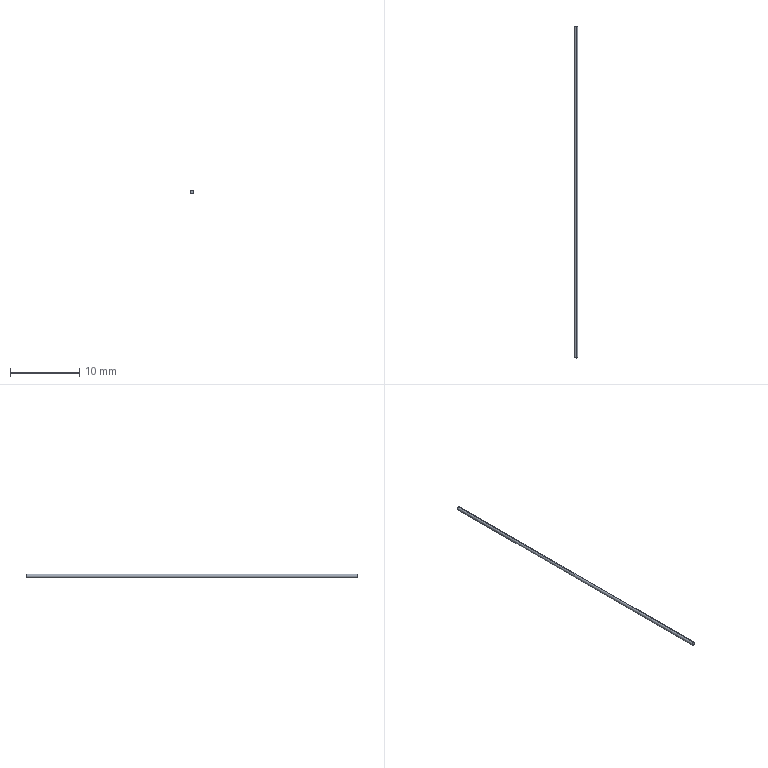Part | SolidWorks | features Revolution 1 | 1 solid | 4 faces | box 0.5 x 48 x 0.5 mm | volume 9.425 mm3 | cylinder 2 | plane 2 | commonest cylinder face diameters 0.5 x2
STEP:
#1=CARTESIAN_POINT('',(0.,48.,-0.25));
#2=VERTEX_POINT('',#1);
#3=CARTESIAN_POINT('',(0.,48.,0.25));
#4=VERTEX_POINT('',#3);
#5=CARTESIAN_POINT('',(0.,48.,0.));
#6=DIRECTION('',(0.,-1.,0.));
#7=DIRECTION('',(0.,0.,-1.));
#8=AXIS2_PLACEMENT_3D('',#5,#6,#7);
#9=CIRCLE('',#8,0.25);
#10=EDGE_CURVE('',#2,#4,#9,.T.);
#11=ORIENTED_EDGE('',*,*,#10,.T.);
#12=CARTESIAN_POINT('',(0.,0.,0.25));
#13=VERTEX_POINT('',#12);
#14=CARTESIAN_POINT('',(0.,0.,0.25));
#15=DIRECTION('',(0.,-1.,0.));
#16=VECTOR('',#15,1000.);
#17=LINE('',#14,#16);
#18=EDGE_CURVE('',#4,#13,#17,.T.);
#19=ORIENTED_EDGE('',*,*,#18,.T.);
#20=CARTESIAN_POINT('',(0.,0.,-0.25));
#21=VERTEX_POINT('',#20);
#22=CARTESIAN_POINT('',(0.,0.,0.));
#23=DIRECTION('',(0.,-1.,0.));
#24=DIRECTION('',(0.,0.,-1.));
#25=AXIS2_PLACEMENT_3D('',#22,#23,#24);
#26=CIRCLE('',#25,0.25);
#27=EDGE_CURVE('',#21,#13,#26,.T.);
#28=ORIENTED_EDGE('',*,*,#27,.F.);
#29=CARTESIAN_POINT('',(0.,0.,-0.25));
#30=DIRECTION('',(0.,-1.,0.));
#31=VECTOR('',#30,1000.);
#32=LINE('',#29,#31);
#33=EDGE_CURVE('',#2,#21,#32,.T.);
#34=ORIENTED_EDGE('',*,*,#33,.F.);
#35=EDGE_LOOP('',(#11,#19,#28,#34));
#36=FACE_OUTER_BOUND('',#35,.T.);
#37=CARTESIAN_POINT('',(0.,0.,0.));
#38=DIRECTION('',(0.,-1.,0.));
#39=DIRECTION('',(0.,0.,-1.));
#40=AXIS2_PLACEMENT_3D('',#37,#38,#39);
#41=CYLINDRICAL_SURFACE('',#40,0.25);
#42=ADVANCED_FACE('',(#36),#41,.T.);
#43=ORIENTED_EDGE('',*,*,#10,.F.);
#44=CARTESIAN_POINT('',(0.,48.,0.));
#45=DIRECTION('',(0.,-1.,0.));
#46=DIRECTION('',(0.,0.,-1.));
#47=AXIS2_PLACEMENT_3D('',#44,#45,#46);
#48=CIRCLE('',#47,0.25);
#49=EDGE_CURVE('',#4,#2,#48,.T.);
#50=ORIENTED_EDGE('',*,*,#49,.F.);
#51=EDGE_LOOP('',(#43,#50));
#52=FACE_OUTER_BOUND('',#51,.T.);
#53=CARTESIAN_POINT('',(0.,48.,0.));
#54=DIRECTION('',(0.,-1.,0.));
#55=DIRECTION('',(0.,0.,-1.));
#56=AXIS2_PLACEMENT_3D('',#53,#54,#55);
#57=PLANE('',#56);
#58=ADVANCED_FACE('',(#52),#57,.F.);
#59=ORIENTED_EDGE('',*,*,#18,.F.);
#60=ORIENTED_EDGE('',*,*,#49,.T.);
#61=ORIENTED_EDGE('',*,*,#33,.T.);
#62=CARTESIAN_POINT('',(0.,0.,0.));
#63=DIRECTION('',(0.,-1.,0.));
#64=DIRECTION('',(0.,0.,-1.));
#65=AXIS2_PLACEMENT_3D('',#62,#63,#64);
#66=CIRCLE('',#65,0.25);
#67=EDGE_CURVE('',#13,#21,#66,.T.);
#68=ORIENTED_EDGE('',*,*,#67,.F.);
#69=EDGE_LOOP('',(#59,#60,#61,#68));
#70=FACE_OUTER_BOUND('',#69,.T.);
#71=CARTESIAN_POINT('',(0.,0.,0.));
#72=DIRECTION('',(0.,-1.,0.));
#73=DIRECTION('',(0.,0.,-1.));
#74=AXIS2_PLACEMENT_3D('',#71,#72,#73);
#75=CYLINDRICAL_SURFACE('',#74,0.25);
#76=ADVANCED_FACE('',(#70),#75,.T.);
#77=ORIENTED_EDGE('',*,*,#27,.T.);
#78=ORIENTED_EDGE('',*,*,#67,.T.);
#79=EDGE_LOOP('',(#77,#78));
#80=FACE_OUTER_BOUND('',#79,.T.);
#81=CARTESIAN_POINT('',(0.,0.,0.));
#82=DIRECTION('',(0.,1.,0.));
#83=DIRECTION('',(0.,0.,1.));
#84=AXIS2_PLACEMENT_3D('',#81,#82,#83);
#85=PLANE('',#84);
#86=ADVANCED_FACE('',(#80),#85,.F.);
#87=CLOSED_SHELL('',(#42,#58,#76,#86));
#88=MANIFOLD_SOLID_BREP('',#87);
#89=CARTESIAN_POINT('',(0.,0.,0.));
#90=DIRECTION('',(0.,0.,1.));
#91=DIRECTION('',(1.,0.,0.));
#92=AXIS2_PLACEMENT_3D('',#89,#90,#91);
#93=(LENGTH_UNIT()NAMED_UNIT(*)SI_UNIT(.MILLI.,.METRE.));
#94=UNCERTAINTY_MEASURE_WITH_UNIT(LENGTH_MEASURE(0.00001),#93,'','');
#95=(NAMED_UNIT(*)PLANE_ANGLE_UNIT()SI_UNIT($,.RADIAN.));
#96=(NAMED_UNIT(*)SI_UNIT($,.STERADIAN.)SOLID_ANGLE_UNIT());
#97=(GEOMETRIC_REPRESENTATION_CONTEXT(3)GLOBAL_UNCERTAINTY_ASSIGNED_CONTEXT((#94))GLOBAL_UNIT_ASSIGNED_CONTEXT((#93,#95,#96))REPRESENTATION_CONTEXT('',''));
#98=ADVANCED_BREP_SHAPE_REPRESENTATION('',(#88,#92),#97);